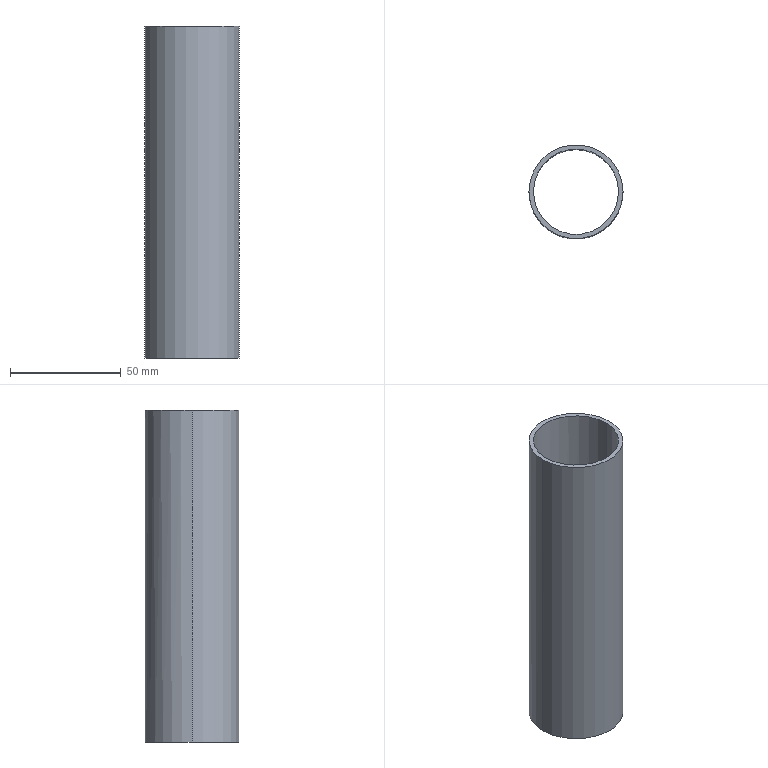Part | NX | features MYKP38-240_3 2 | 1 solid | 6 faces | box 42.5 x 42.5 x 150 mm | volume 38170 mm3 | cylinder 4 | plane 2 | commonest cylinder face diameters 38.5 x2 42.5 x2
STEP:
#1=CARTESIAN_POINT('',(-441.273,281.595,-8.87));
#2=VERTEX_POINT('',#1);
#3=CARTESIAN_POINT('',(-420.023,302.845,-8.87));
#4=VERTEX_POINT('',#3);
#5=CARTESIAN_POINT('',(-420.023,281.595,-8.87));
#6=DIRECTION('',(0.,0.,-1.));
#7=DIRECTION('',(-1.,0.,0.));
#8=AXIS2_PLACEMENT_3D('',#5,#6,#7);
#9=CIRCLE('',#8,21.25);
#10=EDGE_CURVE('',#2,#4,#9,.T.);
#11=ORIENTED_EDGE('',*,*,#10,.T.);
#12=CARTESIAN_POINT('',(-398.773,281.595,-8.87));
#13=VERTEX_POINT('',#12);
#14=CARTESIAN_POINT('',(-420.023,281.595,-8.87));
#15=DIRECTION('',(0.,0.,-1.));
#16=DIRECTION('',(0.,1.,0.));
#17=AXIS2_PLACEMENT_3D('',#14,#15,#16);
#18=CIRCLE('',#17,21.25);
#19=EDGE_CURVE('',#4,#13,#18,.T.);
#20=ORIENTED_EDGE('',*,*,#19,.T.);
#21=CARTESIAN_POINT('',(-420.023,281.595,-8.87));
#22=DIRECTION('',(0.,0.,-1.));
#23=DIRECTION('',(1.,0.,0.));
#24=AXIS2_PLACEMENT_3D('',#21,#22,#23);
#25=CIRCLE('',#24,21.25);
#26=EDGE_CURVE('',#13,#2,#25,.T.);
#27=ORIENTED_EDGE('',*,*,#26,.T.);
#28=EDGE_LOOP('',(#11,#20,#27));
#29=FACE_BOUND('',#28,.T.);
#30=CARTESIAN_POINT('',(-420.023,300.845,-8.87));
#31=VERTEX_POINT('',#30);
#32=CARTESIAN_POINT('',(-439.273,281.595,-8.87));
#33=VERTEX_POINT('',#32);
#34=CARTESIAN_POINT('',(-420.023,281.595,-8.87));
#35=DIRECTION('',(0.,0.,1.));
#36=DIRECTION('',(0.,1.,0.));
#37=AXIS2_PLACEMENT_3D('',#34,#35,#36);
#38=CIRCLE('',#37,19.25);
#39=EDGE_CURVE('',#31,#33,#38,.T.);
#40=ORIENTED_EDGE('',*,*,#39,.T.);
#41=CARTESIAN_POINT('',(-420.023,262.345,-8.87));
#42=VERTEX_POINT('',#41);
#43=CARTESIAN_POINT('',(-420.023,281.595,-8.87));
#44=DIRECTION('',(0.,0.,1.));
#45=DIRECTION('',(-1.,0.,0.));
#46=AXIS2_PLACEMENT_3D('',#43,#44,#45);
#47=CIRCLE('',#46,19.25);
#48=EDGE_CURVE('',#33,#42,#47,.T.);
#49=ORIENTED_EDGE('',*,*,#48,.T.);
#50=CARTESIAN_POINT('',(-400.773,281.595,-8.87));
#51=VERTEX_POINT('',#50);
#52=CARTESIAN_POINT('',(-420.023,281.595,-8.87));
#53=DIRECTION('',(0.,0.,1.));
#54=DIRECTION('',(0.,-1.,0.));
#55=AXIS2_PLACEMENT_3D('',#52,#53,#54);
#56=CIRCLE('',#55,19.25);
#57=EDGE_CURVE('',#42,#51,#56,.T.);
#58=ORIENTED_EDGE('',*,*,#57,.T.);
#59=CARTESIAN_POINT('',(-420.023,281.595,-8.87));
#60=DIRECTION('',(0.,0.,1.));
#61=DIRECTION('',(1.,0.,0.));
#62=AXIS2_PLACEMENT_3D('',#59,#60,#61);
#63=CIRCLE('',#62,19.25);
#64=EDGE_CURVE('',#51,#31,#63,.T.);
#65=ORIENTED_EDGE('',*,*,#64,.T.);
#66=EDGE_LOOP('',(#40,#49,#58,#65));
#67=FACE_BOUND('',#66,.T.);
#68=CARTESIAN_POINT('',(-420.023,305.345,-8.87));
#69=DIRECTION('',(0.,0.,1.));
#70=DIRECTION('',(1.,0.,0.));
#71=AXIS2_PLACEMENT_3D('',#68,#69,#70);
#72=PLANE('',#71);
#73=ADVANCED_FACE('',(#29,#67),#72,.F.);
#74=CARTESIAN_POINT('',(-441.273,281.595,141.13));
#75=VERTEX_POINT('',#74);
#76=CARTESIAN_POINT('',(-441.273,281.595,31.13));
#77=DIRECTION('',(0.,0.,-1.));
#78=VECTOR('',#77,1000.);
#79=LINE('',#76,#78);
#80=EDGE_CURVE('',#2,#75,#79,.F.);
#81=ORIENTED_EDGE('',*,*,#80,.F.);
#82=ORIENTED_EDGE('',*,*,#26,.F.);
#83=CARTESIAN_POINT('',(-398.773,281.595,141.13));
#84=VERTEX_POINT('',#83);
#85=CARTESIAN_POINT('',(-398.773,281.595,-3952.87));
#86=DIRECTION('',(0.,0.,-1.));
#87=VECTOR('',#86,1000.);
#88=LINE('',#85,#87);
#89=EDGE_CURVE('',#84,#13,#88,.T.);
#90=ORIENTED_EDGE('',*,*,#89,.F.);
#91=CARTESIAN_POINT('',(-420.023,281.595,141.13));
#92=DIRECTION('',(0.,0.,1.));
#93=DIRECTION('',(-1.,0.,0.));
#94=AXIS2_PLACEMENT_3D('',#91,#92,#93);
#95=CIRCLE('',#94,21.25);
#96=EDGE_CURVE('',#75,#84,#95,.T.);
#97=ORIENTED_EDGE('',*,*,#96,.F.);
#98=EDGE_LOOP('',(#81,#82,#90,#97));
#99=FACE_BOUND('',#98,.T.);
#100=CARTESIAN_POINT('',(-420.023,281.595,191.13));
#101=DIRECTION('',(0.,0.,-1.));
#102=DIRECTION('',(0.,1.,0.));
#103=AXIS2_PLACEMENT_3D('',#100,#101,#102);
#104=CYLINDRICAL_SURFACE('',#103,21.25);
#105=ADVANCED_FACE('',(#99),#104,.T.);
#106=CARTESIAN_POINT('',(-439.273,281.595,141.13));
#107=VERTEX_POINT('',#106);
#108=CARTESIAN_POINT('',(-439.273,281.595,31.13));
#109=DIRECTION('',(0.,0.,-1.));
#110=VECTOR('',#109,1000.);
#111=LINE('',#108,#110);
#112=EDGE_CURVE('',#33,#107,#111,.F.);
#113=ORIENTED_EDGE('',*,*,#112,.F.);
#114=ORIENTED_EDGE('',*,*,#39,.F.);
#115=ORIENTED_EDGE('',*,*,#64,.F.);
#116=CARTESIAN_POINT('',(-400.773,281.595,141.13));
#117=VERTEX_POINT('',#116);
#118=CARTESIAN_POINT('',(-400.773,281.595,-3952.87));
#119=DIRECTION('',(0.,0.,-1.));
#120=VECTOR('',#119,1000.);
#121=LINE('',#118,#120);
#122=EDGE_CURVE('',#117,#51,#121,.T.);
#123=ORIENTED_EDGE('',*,*,#122,.F.);
#124=CARTESIAN_POINT('',(-420.023,281.595,141.13));
#125=DIRECTION('',(0.,0.,-1.));
#126=DIRECTION('',(-1.,0.,0.));
#127=AXIS2_PLACEMENT_3D('',#124,#125,#126);
#128=CIRCLE('',#127,19.25);
#129=EDGE_CURVE('',#107,#117,#128,.T.);
#130=ORIENTED_EDGE('',*,*,#129,.F.);
#131=EDGE_LOOP('',(#113,#114,#115,#123,#130));
#132=FACE_BOUND('',#131,.T.);
#133=CARTESIAN_POINT('',(-420.023,281.595,191.13));
#134=DIRECTION('',(0.,0.,-1.));
#135=DIRECTION('',(0.,1.,0.));
#136=AXIS2_PLACEMENT_3D('',#133,#134,#135);
#137=CYLINDRICAL_SURFACE('',#136,19.25);
#138=ADVANCED_FACE('',(#132),#137,.F.);
#139=ORIENTED_EDGE('',*,*,#89,.T.);
#140=ORIENTED_EDGE('',*,*,#19,.F.);
#141=ORIENTED_EDGE('',*,*,#10,.F.);
#142=ORIENTED_EDGE('',*,*,#80,.T.);
#143=CARTESIAN_POINT('',(-420.023,281.595,141.13));
#144=DIRECTION('',(0.,0.,1.));
#145=DIRECTION('',(1.,0.,0.));
#146=AXIS2_PLACEMENT_3D('',#143,#144,#145);
#147=CIRCLE('',#146,21.25);
#148=EDGE_CURVE('',#84,#75,#147,.T.);
#149=ORIENTED_EDGE('',*,*,#148,.F.);
#150=EDGE_LOOP('',(#139,#140,#141,#142,#149));
#151=FACE_BOUND('',#150,.T.);
#152=CARTESIAN_POINT('',(-420.023,281.595,191.13));
#153=DIRECTION('',(0.,0.,-1.));
#154=DIRECTION('',(0.,1.,0.));
#155=AXIS2_PLACEMENT_3D('',#152,#153,#154);
#156=CYLINDRICAL_SURFACE('',#155,21.25);
#157=ADVANCED_FACE('',(#151),#156,.T.);
#158=ORIENTED_EDGE('',*,*,#122,.T.);
#159=ORIENTED_EDGE('',*,*,#57,.F.);
#160=ORIENTED_EDGE('',*,*,#48,.F.);
#161=ORIENTED_EDGE('',*,*,#112,.T.);
#162=CARTESIAN_POINT('',(-420.023,281.595,141.13));
#163=DIRECTION('',(0.,0.,-1.));
#164=DIRECTION('',(1.,0.,0.));
#165=AXIS2_PLACEMENT_3D('',#162,#163,#164);
#166=CIRCLE('',#165,19.25);
#167=EDGE_CURVE('',#117,#107,#166,.T.);
#168=ORIENTED_EDGE('',*,*,#167,.F.);
#169=EDGE_LOOP('',(#158,#159,#160,#161,#168));
#170=FACE_BOUND('',#169,.T.);
#171=CARTESIAN_POINT('',(-420.023,281.595,191.13));
#172=DIRECTION('',(0.,0.,-1.));
#173=DIRECTION('',(0.,1.,0.));
#174=AXIS2_PLACEMENT_3D('',#171,#172,#173);
#175=CYLINDRICAL_SURFACE('',#174,19.25);
#176=ADVANCED_FACE('',(#170),#175,.F.);
#177=ORIENTED_EDGE('',*,*,#148,.T.);
#178=ORIENTED_EDGE('',*,*,#96,.T.);
#179=EDGE_LOOP('',(#177,#178));
#180=FACE_BOUND('',#179,.T.);
#181=ORIENTED_EDGE('',*,*,#167,.T.);
#182=ORIENTED_EDGE('',*,*,#129,.T.);
#183=EDGE_LOOP('',(#181,#182));
#184=FACE_BOUND('',#183,.T.);
#185=CARTESIAN_POINT('',(-420.023,318.095,141.13));
#186=DIRECTION('',(0.,0.,-1.));
#187=DIRECTION('',(0.,-1.,0.));
#188=AXIS2_PLACEMENT_3D('',#185,#186,#187);
#189=PLANE('',#188);
#190=ADVANCED_FACE('',(#180,#184),#189,.F.);
#191=CLOSED_SHELL('',(#73,#105,#138,#157,#176,#190));
#192=MANIFOLD_SOLID_BREP('',#191);
#193=(LENGTH_UNIT()NAMED_UNIT(*)SI_UNIT(.MILLI.,.METRE.));
#194=UNCERTAINTY_MEASURE_WITH_UNIT(LENGTH_MEASURE(0.00001),#193,'','');
#195=(NAMED_UNIT(*)PLANE_ANGLE_UNIT()SI_UNIT($,.RADIAN.));
#196=(NAMED_UNIT(*)SI_UNIT($,.STERADIAN.)SOLID_ANGLE_UNIT());
#197=(GEOMETRIC_REPRESENTATION_CONTEXT(3)GLOBAL_UNCERTAINTY_ASSIGNED_CONTEXT((#194))GLOBAL_UNIT_ASSIGNED_CONTEXT((#193,#195,#196))REPRESENTATION_CONTEXT('',''));
#198=ADVANCED_BREP_SHAPE_REPRESENTATION('',(#192),#197);